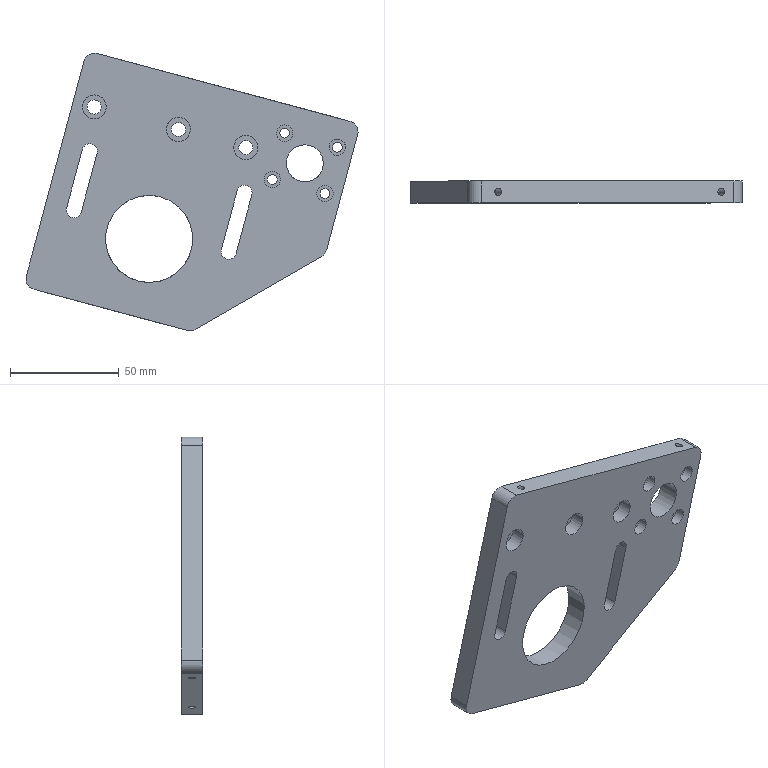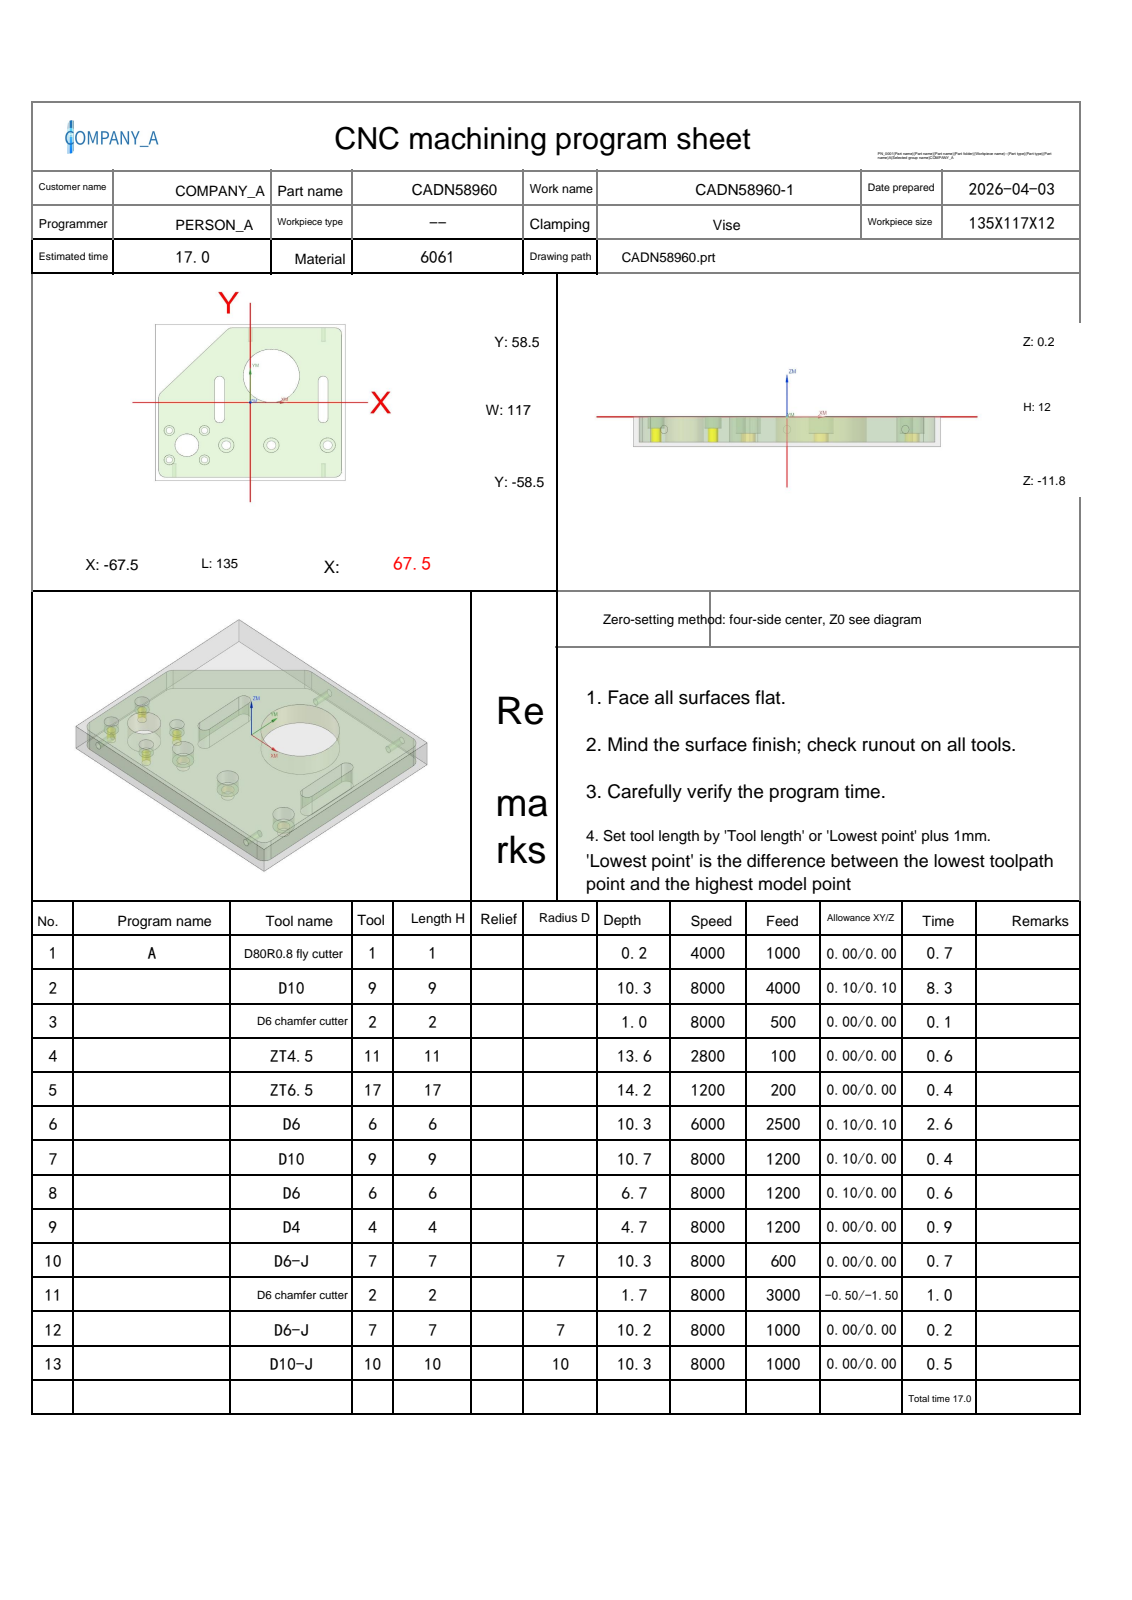NC program | NX | posted by the shop | part box 152.311 x 10 x 127.359 mm
Lines 3046 to 4827 of 4827, first 1275 of 1782 lines:
N3 T02 M06
(D6 chamfer cutter  D=6. R=0. H=02 ce=0.00 di=0.10)
G00 G90 G54 X15. Y19.989 M03 S8000
G43 H02 Z20.
M08
G98 G82 X15. Y19.989 Z-.8 R1. F500.
G80
G00 Z20.
G00 G90 X55. Y-32. M03 S8000
Z20.
G98 G81 X55. Y-32. Z-.8 R1. F500.
X15.
X-17.
X-32.5 Y-21.
Y-43.
X-45. Y-32.
X-57.5 Y-21.
Y-43.
G80
G00 Z20.
G91 G28 Z0.0
M05
M09
G91 G28 Z0.0
M01
N4 T11 M06
(ZT4.5 D=4.5 DR_a=118 H=11)
G00 G90 G54 X-57.5 Y-21. M03 S2800
G43 H11 Z20.
M08
G98 G83 X-57.5 Y-21. Z-13.352 R1. F100. Q2.
Y-43.
X-32.5
Y-21.
G80
G00 Z20.
G91 G28 Z0.0
M05
M09
G91 G28 Z0.0
M01
N5 T17 M06
(ZT6.5 D=6.5 DR_a=118 H=17)
G00 G90 G54 X55. Y-32. M03 S1200
G43 H17 Z20.
M08
G98 G83 X55. Y-32. Z-13.953 R1. F150. Q2.
X15.
X-17.
G80
G00 Z20.
G00 G90 X-45. Y-32. M03 S800
Z20.
G98 G83 X-45. Y-32. Z-13.953 R1. F200. Q3.
G80
G00 Z20.
G91 G28 Z0.0
M05
M09
G91 G28 Z0.0
M01
N6 T06 M06
(D6  D=6. R=0. H=06 ce=0.10 di=0.10)
G00 G90 G54 X51.37 Y2.219 M03 S6000
G43 H06 Z20.
M08
Z.5
G01 Y-11.781 Z.453 F2500.
G03 X51.77 Y-12.181 Z.451 I.4 J0.0
X52.169 Y-11.781 Z.449 I0.0 J.4
G01 Y16.219 Z.355
G03 X51.875 Y16.605 Z.353 I-.4 J0.0
G01 X51.824 Y16.625
X51.77 Y16.619
G03 X51.37 Y16.219 Z.351 I0.0 J-.4
G01 Y-11.781 Z.257
G03 X51.77 Y-12.181 Z.255 I.4 J0.0
X52.169 Y-11.781 Z.253 I0.0 J.4
G01 Y16.219 Z.159
G03 X51.875 Y16.605 Z.157 I-.4 J0.0
G01 X51.824 Y16.625
X51.77 Y16.619 Z.156
G03 X51.37 Y16.219 Z.154 I0.0 J-.4
G01 Y-11.781 Z.06
G03 X51.77 Y-12.181 Z.058 I.4 J0.0
X52.169 Y-11.781 Z.056 I0.0 J.4
G01 Y16.219 Z-.038
G03 X51.875 Y16.605 Z-.039 I-.4 J0.0
G01 X51.824 Y16.625 Z-.04
X51.77 Y16.619
G03 X51.37 Y16.219 Z-.042 I0.0 J-.4
G01 Y-11.781 Z-.136
G03 X51.77 Y-12.181 Z-.138 I.4 J0.0
X52.169 Y-11.781 Z-.14 I0.0 J.4
G01 Y16.219 Z-.234
G03 X51.875 Y16.605 Z-.236 I-.4 J0.0
G01 X51.824 Y16.625
X51.77 Y16.619
G03 X51.37 Y16.219 Z-.238 I0.0 J-.4
G01 Y-11.781 Z-.332
G03 X51.77 Y-12.181 Z-.334 I.4 J0.0
X52.169 Y-11.781 Z-.336 I0.0 J.4
G01 Y16.219 Z-.43
G03 X51.875 Y16.605 Z-.432 I-.4 J0.0
G01 X51.824 Y16.625
X51.77 Y16.619
G03 X51.37 Y16.219 Z-.435 I0.0 J-.4
G01 Y-11.781 Z-.528
G03 X51.77 Y-12.181 Z-.531 I.4 J0.0
X52.169 Y-11.781 Z-.533 I0.0 J.4
G01 Y16.219 Z-.627
G03 X51.875 Y16.605 Z-.628 I-.4 J0.0
G01 X51.824 Y16.625 Z-.629
X51.77 Y16.619
G03 X51.37 Y16.219 Z-.631 I0.0 J-.4
G01 Y-11.781 Z-.725
G03 X51.77 Y-12.181 Z-.727 I.4 J0.0
X52.169 Y-11.781 Z-.729 I0.0 J.4
G01 Y16.219 Z-.823
G03 X51.875 Y16.605 Z-.825 I-.4 J0.0
G01 X51.824 Y16.625
X51.77 Y16.619
G03 X51.37 Y16.219 Z-.827 I0.0 J-.4
G01 Y-11.781 Z-.921
G03 X51.77 Y-12.181 Z-.923 I.4 J0.0
X52.169 Y-11.781 Z-.925 I0.0 J.4
G01 Y16.219 Z-1.019
G03 X51.875 Y16.605 Z-1.021 I-.4 J0.0
G01 X51.824 Y16.625
X51.77 Y16.619
G03 X51.37 Y16.219 Z-1.023 I0.0 J-.4
G01 Y-11.781 Z-1.117
G03 X51.77 Y-12.181 Z-1.119 I.4 J0.0
X52.169 Y-11.781 Z-1.122 I0.0 J.4
G01 Y16.219 Z-1.215
G03 X51.875 Y16.605 Z-1.217 I-.4 J0.0
G01 X51.824 Y16.625
X51.77 Y16.619 Z-1.218
G03 X51.37 Y16.219 Z-1.22 I0.0 J-.4
G01 Y-11.781 Z-1.314
G03 X51.77 Y-12.181 Z-1.316 I.4 J0.0
X52.169 Y-11.781 Z-1.318 I0.0 J.4
G01 Y16.219 Z-1.412
G03 X51.875 Y16.605 Z-1.414 I-.4 J0.0
G01 X51.824 Y16.625
X51.77 Y16.619
G03 X51.37 Y16.219 Z-1.416 I0.0 J-.4
G01 Y-11.781 Z-1.51
G03 X51.77 Y-12.181 Z-1.512 I.4 J0.0
X52.169 Y-11.781 Z-1.514 I0.0 J.4
G01 Y16.219 Z-1.608
G03 X51.875 Y16.605 Z-1.61 I-.4 J0.0
G01 X51.824 Y16.625
X51.77 Y16.619
G03 X51.37 Y16.219 Z-1.612 I0.0 J-.4
G01 Y-11.781 Z-1.706
G03 X51.77 Y-12.181 Z-1.708 I.4 J0.0
X52.169 Y-11.781 Z-1.71 I0.0 J.4
G01 Y16.219 Z-1.804
G03 X51.875 Y16.605 Z-1.806 I-.4 J0.0
G01 X51.824 Y16.625
X51.77 Y16.619
G03 X51.37 Y16.219 Z-1.809 I0.0 J-.4
G01 Y-11.781 Z-1.903
G03 X51.77 Y-12.181 Z-1.905 I.4 J0.0
X52.169 Y-11.781 Z-1.907 I0.0 J.4
G01 Y16.219 Z-2.001
G03 X51.875 Y16.605 Z-2.002 I-.4 J0.0
G01 X51.824 Y16.625 Z-2.003
X51.77 Y16.619
G03 X51.37 Y16.219 Z-2.005 I0.0 J-.4
G01 Y-11.781 Z-2.099
G03 X51.77 Y-12.181 Z-2.101 I.4 J0.0
X52.169 Y-11.781 Z-2.103 I0.0 J.4
G01 Y16.219 Z-2.197
G03 X51.875 Y16.605 Z-2.199 I-.4 J0.0
G01 X51.824 Y16.625
X51.77 Y16.619
G03 X51.37 Y16.219 Z-2.201 I0.0 J-.4
G01 Y-11.781 Z-2.295
G03 X51.77 Y-12.181 Z-2.297 I.4 J0.0
X52.169 Y-11.781 Z-2.299 I0.0 J.4
G01 Y16.219 Z-2.393
G03 X51.875 Y16.605 Z-2.395 I-.4 J0.0
G01 X51.824 Y16.625
X51.77 Y16.619
G03 X51.37 Y16.219 Z-2.397 I0.0 J-.4
G01 Y-11.781 Z-2.491
G03 X51.77 Y-12.181 Z-2.494 I.4 J0.0
X52.169 Y-11.781 Z-2.496 I0.0 J.4
G01 Y16.219 Z-2.59
G03 X51.875 Y16.605 Z-2.591 I-.4 J0.0
G01 X51.824 Y16.625
X51.77 Y16.619 Z-2.592
G03 X51.37 Y16.219 Z-2.594 I0.0 J-.4
G01 Y-11.781 Z-2.688
G03 X51.77 Y-12.181 Z-2.69 I.4 J0.0
X52.169 Y-11.781 Z-2.692 I0.0 J.4
G01 Y16.219 Z-2.786
G03 X51.875 Y16.605 Z-2.788 I-.4 J0.0
G01 X51.824 Y16.625
X51.77 Y16.619
G03 X51.37 Y16.219 Z-2.79 I0.0 J-.4
G01 Y-11.781 Z-2.884
G03 X51.77 Y-12.181 Z-2.886 I.4 J0.0
X52.169 Y-11.781 Z-2.888 I0.0 J.4
G01 Y16.219 Z-2.982
G03 X51.875 Y16.605 Z-2.984 I-.4 J0.0
G01 X51.824 Y16.625
X51.77 Y16.619
G03 X51.37 Y16.219 Z-2.986 I0.0 J-.4
G01 Y-11.781 Z-3.08
G03 X51.77 Y-12.181 Z-3.082 I.4 J0.0
X52.169 Y-11.781 Z-3.085 I0.0 J.4
G01 Y16.219 Z-3.178
G03 X51.875 Y16.605 Z-3.18 I-.4 J0.0
G01 X51.824 Y16.625
X51.77 Y16.619 Z-3.181
G03 X51.37 Y16.219 Z-3.183 I0.0 J-.4
G01 Y-11.781 Z-3.277
G03 X51.77 Y-12.181 Z-3.279 I.4 J0.0
X52.169 Y-11.781 Z-3.281 I0.0 J.4
G01 Y16.219 Z-3.375
G03 X51.875 Y16.605 Z-3.376 I-.4 J0.0
G01 X51.824 Y16.625 Z-3.377
X51.77 Y16.619
G03 X51.37 Y16.219 Z-3.379 I0.0 J-.4
G01 Y-11.781 Z-3.473
G03 X51.77 Y-12.181 Z-3.475 I.4 J0.0
X52.169 Y-11.781 Z-3.477 I0.0 J.4
G01 Y16.219 Z-3.571
G03 X51.875 Y16.605 Z-3.573 I-.4 J0.0
G01 X51.824 Y16.625
X51.77 Y16.619
G03 X51.37 Y16.219 Z-3.575 I0.0 J-.4
G01 Y-11.781 Z-3.669
G03 X51.77 Y-12.181 Z-3.671 I.4 J0.0
X52.169 Y-11.781 Z-3.673 I0.0 J.4
G01 Y16.219 Z-3.767
G03 X51.875 Y16.605 Z-3.769 I-.4 J0.0
G01 X51.824 Y16.625
X51.77 Y16.619
G03 X51.37 Y16.219 Z-3.772 I0.0 J-.4
G01 Y-11.781 Z-3.865
G03 X51.77 Y-12.181 Z-3.868 I.4 J0.0
X52.169 Y-11.781 Z-3.87 I0.0 J.4
G01 Y16.219 Z-3.964
G03 X51.875 Y16.605 Z-3.965 I-.4 J0.0
G01 X51.824 Y16.625 Z-3.966
X51.77 Y16.619
G03 X51.37 Y16.219 Z-3.968 I0.0 J-.4
G01 Y-11.781 Z-4.062
G03 X51.77 Y-12.181 Z-4.064 I.4 J0.0
X52.169 Y-11.781 Z-4.066 I0.0 J.4
G01 Y16.219 Z-4.16
G03 X51.875 Y16.605 Z-4.162 I-.4 J0.0
G01 X51.824 Y16.625
X51.77 Y16.619
G03 X51.37 Y16.219 Z-4.164 I0.0 J-.4
G01 Y-11.781 Z-4.258
G03 X51.77 Y-12.181 Z-4.26 I.4 J0.0
X52.169 Y-11.781 Z-4.262 I0.0 J.4
G01 Y16.219 Z-4.356
G03 X51.875 Y16.605 Z-4.358 I-.4 J0.0
G01 X51.824 Y16.625
X51.77 Y16.619
G03 X51.37 Y16.219 Z-4.36 I0.0 J-.4
G01 Y-11.781 Z-4.454
G03 X51.77 Y-12.181 Z-4.456 I.4 J0.0
X52.169 Y-11.781 Z-4.459 I0.0 J.4
G01 Y16.219 Z-4.553
G03 X51.875 Y16.605 Z-4.554 I-.4 J0.0
G01 X51.824 Y16.625
X51.77 Y16.619 Z-4.555
G03 X51.37 Y16.219 Z-4.557 I0.0 J-.4
G01 Y-11.781 Z-4.651
G03 X51.77 Y-12.181 Z-4.653 I.4 J0.0
X52.169 Y-11.781 Z-4.655 I0.0 J.4
G01 Y16.219 Z-4.749
G03 X51.875 Y16.605 Z-4.751 I-.4 J0.0
G01 X51.824 Y16.625
X51.77 Y16.619
G03 X51.37 Y16.219 Z-4.753 I0.0 J-.4
G01 Y-11.781 Z-4.847
G03 X51.77 Y-12.181 Z-4.849 I.4 J0.0
X52.169 Y-11.781 Z-4.851 I0.0 J.4
G01 Y16.219 Z-4.945
G03 X51.875 Y16.605 Z-4.947 I-.4 J0.0
G01 X51.824 Y16.625
X51.77 Y16.619
G03 X51.37 Y16.219 Z-4.949 I0.0 J-.4
G01 Y-11.781 Z-5.043
G03 X51.77 Y-12.181 Z-5.045 I.4 J0.0
X52.169 Y-11.781 Z-5.047 I0.0 J.4
G01 Y16.219 Z-5.141
G03 X51.875 Y16.605 Z-5.143 I-.4 J0.0
G01 X51.824 Y16.625
X51.77 Y16.619 Z-5.144
G03 X51.37 Y16.219 Z-5.146 I0.0 J-.4
G01 Y-11.781 Z-5.24
G03 X51.77 Y-12.181 Z-5.242 I.4 J0.0
X52.169 Y-11.781 Z-5.244 I0.0 J.4
G01 Y16.219 Z-5.338
G03 X51.875 Y16.605 Z-5.339 I-.4 J0.0
G01 X51.824 Y16.625 Z-5.34
X51.77 Y16.619
G03 X51.37 Y16.219 Z-5.342 I0.0 J-.4
G01 Y-11.781 Z-5.436
G03 X51.77 Y-12.181 Z-5.438 I.4 J0.0
X52.169 Y-11.781 Z-5.44 I0.0 J.4
G01 Y16.219 Z-5.534
G03 X51.875 Y16.605 Z-5.536 I-.4 J0.0
G01 X51.824 Y16.625
X51.77 Y16.619
G03 X51.37 Y16.219 Z-5.538 I0.0 J-.4
G01 Y-11.781 Z-5.632
G03 X51.77 Y-12.181 Z-5.634 I.4 J0.0
X52.169 Y-11.781 Z-5.636 I0.0 J.4
G01 Y16.219 Z-5.73
G03 X51.875 Y16.605 Z-5.732 I-.4 J0.0
G01 X51.824 Y16.625
X51.77 Y16.619
G03 X51.37 Y16.219 Z-5.735 I0.0 J-.4
G01 Y-11.781 Z-5.828
G03 X51.77 Y-12.181 Z-5.831 I.4 J0.0
X52.169 Y-11.781 Z-5.833 I0.0 J.4
G01 Y16.219 Z-5.927
G03 X51.875 Y16.605 Z-5.928 I-.4 J0.0
G01 X51.824 Y16.625 Z-5.929
X51.77 Y16.619
G03 X51.37 Y16.219 Z-5.931 I0.0 J-.4
G01 Y-11.781 Z-6.025
G03 X51.77 Y-12.181 Z-6.027 I.4 J0.0
X52.169 Y-11.781 Z-6.029 I0.0 J.4
G01 Y16.219 Z-6.123
G03 X51.875 Y16.605 Z-6.125 I-.4 J0.0
G01 X51.824 Y16.625
X51.77 Y16.619
G03 X51.37 Y16.219 Z-6.127 I0.0 J-.4
G01 Y-11.781 Z-6.221
G03 X51.77 Y-12.181 Z-6.223 I.4 J0.0
X52.169 Y-11.781 Z-6.225 I0.0 J.4
G01 Y16.219 Z-6.319
G03 X51.875 Y16.605 Z-6.321 I-.4 J0.0
G01 X51.824 Y16.625
X51.77 Y16.619
G03 X51.37 Y16.219 Z-6.323 I0.0 J-.4
G01 Y-11.781 Z-6.417
G03 X51.77 Y-12.181 Z-6.419 I.4 J0.0
X52.169 Y-11.781 Z-6.422 I0.0 J.4
G01 Y16.219 Z-6.515
G03 X51.875 Y16.605 Z-6.517 I-.4 J0.0
G01 X51.824 Y16.625
X51.77 Y16.619 Z-6.518
G03 X51.37 Y16.219 Z-6.52 I0.0 J-.4
G01 Y-11.781 Z-6.614
G03 X51.77 Y-12.181 Z-6.616 I.4 J0.0
X52.169 Y-11.781 Z-6.618 I0.0 J.4
G01 Y16.219 Z-6.712
G03 X51.875 Y16.605 Z-6.714 I-.4 J0.0
G01 X51.824 Y16.625
X51.77 Y16.619
G03 X51.37 Y16.219 Z-6.716 I0.0 J-.4
G01 Y-11.781 Z-6.81
G03 X51.77 Y-12.181 Z-6.812 I.4 J0.0
X52.169 Y-11.781 Z-6.814 I0.0 J.4
G01 Y16.219 Z-6.908
G03 X51.875 Y16.605 Z-6.91 I-.4 J0.0
G01 X51.824 Y16.625
X51.77 Y16.619
G03 X51.37 Y16.219 Z-6.912 I0.0 J-.4
G01 Y-11.781 Z-7.006
G03 X51.77 Y-12.181 Z-7.008 I.4 J0.0
X52.169 Y-11.781 Z-7.01 I0.0 J.4
G01 Y16.219 Z-7.104
G03 X51.875 Y16.605 Z-7.106 I-.4 J0.0
G01 X51.824 Y16.625
X51.77 Y16.619
G03 X51.37 Y16.219 Z-7.109 I0.0 J-.4
G01 Y-11.781 Z-7.203
G03 X51.77 Y-12.181 Z-7.205 I.4 J0.0
X52.169 Y-11.781 Z-7.207 I0.0 J.4
G01 Y16.219 Z-7.301
G03 X51.875 Y16.605 Z-7.302 I-.4 J0.0
G01 X51.824 Y16.625 Z-7.303
X51.77 Y16.619
G03 X51.37 Y16.219 Z-7.305 I0.0 J-.4
G01 Y-11.781 Z-7.399
G03 X51.77 Y-12.181 Z-7.401 I.4 J0.0
X52.169 Y-11.781 Z-7.403 I0.0 J.4
G01 Y16.219 Z-7.497
G03 X51.875 Y16.605 Z-7.499 I-.4 J0.0
G01 X51.824 Y16.625
X51.77 Y16.619
G03 X51.37 Y16.219 Z-7.501 I0.0 J-.4
G01 Y-11.781 Z-7.595
G03 X51.77 Y-12.181 Z-7.597 I.4 J0.0
X52.169 Y-11.781 Z-7.599 I0.0 J.4
G01 Y16.219 Z-7.693
G03 X51.875 Y16.605 Z-7.695 I-.4 J0.0
G01 X51.824 Y16.625
X51.77 Y16.619
G03 X51.37 Y16.219 Z-7.697 I0.0 J-.4
G01 Y-11.781 Z-7.791
G03 X51.77 Y-12.181 Z-7.794 I.4 J0.0
X52.169 Y-11.781 Z-7.796 I0.0 J.4
G01 Y16.219 Z-7.89
G03 X51.875 Y16.605 Z-7.891 I-.4 J0.0
G01 X51.824 Y16.625
X51.77 Y16.619 Z-7.892
G03 X51.37 Y16.219 Z-7.894 I0.0 J-.4
G01 Y-11.781 Z-7.988
G03 X51.77 Y-12.181 Z-7.99 I.4 J0.0
X52.169 Y-11.781 Z-7.992 I0.0 J.4
G01 Y16.219 Z-8.086
G03 X51.875 Y16.605 Z-8.088 I-.4 J0.0
G01 X51.824 Y16.625
X51.77 Y16.619
G03 X51.37 Y16.219 Z-8.09 I0.0 J-.4
G01 Y-11.781 Z-8.184
G03 X51.77 Y-12.181 Z-8.186 I.4 J0.0
X52.169 Y-11.781 Z-8.188 I0.0 J.4
G01 Y16.219 Z-8.282
G03 X51.875 Y16.605 Z-8.284 I-.4 J0.0
G01 X51.824 Y16.625
X51.77 Y16.619
G03 X51.37 Y16.219 Z-8.286 I0.0 J-.4
G01 Y-11.781 Z-8.38
G03 X51.77 Y-12.181 Z-8.382 I.4 J0.0
X52.169 Y-11.781 Z-8.385 I0.0 J.4
G01 Y16.219 Z-8.478
G03 X51.875 Y16.605 Z-8.48 I-.4 J0.0
G01 X51.824 Y16.625
X51.77 Y16.619 Z-8.481
G03 X51.37 Y16.219 Z-8.483 I0.0 J-.4
G01 Y-11.781 Z-8.577
G03 X51.77 Y-12.181 Z-8.579 I.4 J0.0
X52.169 Y-11.781 Z-8.581 I0.0 J.4
G01 Y16.219 Z-8.675
G03 X51.875 Y16.605 Z-8.676 I-.4 J0.0
G01 X51.824 Y16.625 Z-8.677
X51.77 Y16.619
G03 X51.37 Y16.219 Z-8.679 I0.0 J-.4
G01 Y-11.781 Z-8.773
G03 X51.77 Y-12.181 Z-8.775 I.4 J0.0
X52.169 Y-11.781 Z-8.777 I0.0 J.4
G01 Y16.219 Z-8.871
G03 X51.875 Y16.605 Z-8.873 I-.4 J0.0
G01 X51.824 Y16.625
X51.77 Y16.619
G03 X51.37 Y16.219 Z-8.875 I0.0 J-.4
G01 Y-11.781 Z-8.969
G03 X51.77 Y-12.181 Z-8.971 I.4 J0.0
X52.169 Y-11.781 Z-8.973 I0.0 J.4
G01 Y16.219 Z-9.067
G03 X51.875 Y16.605 Z-9.069 I-.4 J0.0
G01 X51.824 Y16.625
X51.77 Y16.619
G03 X51.37 Y16.219 Z-9.072 I0.0 J-.4
G01 Y-11.781 Z-9.165
G03 X51.77 Y-12.181 Z-9.168 I.4 J0.0
X52.169 Y-11.781 Z-9.17 I0.0 J.4
G01 Y16.219 Z-9.264
G03 X51.875 Y16.605 Z-9.265 I-.4 J0.0
G01 X51.824 Y16.625 Z-9.266
X51.77 Y16.619
G03 X51.37 Y16.219 Z-9.268 I0.0 J-.4
G01 Y-11.781 Z-9.362
G03 X51.77 Y-12.181 Z-9.364 I.4 J0.0
X52.169 Y-11.781 Z-9.366 I0.0 J.4
G01 Y16.219 Z-9.46
G03 X51.875 Y16.605 Z-9.462 I-.4 J0.0
G01 X51.824 Y16.625
X51.77 Y16.619
G03 X51.37 Y16.219 Z-9.464 I0.0 J-.4
G01 Y-11.781 Z-9.558
G03 X51.77 Y-12.181 Z-9.56 I.4 J0.0
X52.169 Y-11.781 Z-9.562 I0.0 J.4
G01 Y16.219 Z-9.656
G03 X51.875 Y16.605 Z-9.658 I-.4 J0.0
G01 X51.824 Y16.625
X51.77 Y16.619
G03 X51.37 Y16.219 Z-9.66 I0.0 J-.4
G01 Y-11.781 Z-9.754
G03 X51.77 Y-12.181 Z-9.756 I.4 J0.0
X52.169 Y-11.781 Z-9.759 I0.0 J.4
G01 Y16.219 Z-9.853
G03 X51.875 Y16.605 Z-9.854 I-.4 J0.0
G01 X51.824 Y16.625
X51.77 Y16.619 Z-9.855
G03 X51.37 Y16.219 Z-9.857 I0.0 J-.4
G01 Y-11.781 Z-9.951
G03 X51.77 Y-12.181 Z-9.953 I.4 J0.0
X52.169 Y-11.781 Z-9.955 I0.0 J.4
G01 Y16.219 Z-10.049
G03 X51.875 Y16.605 Z-10.051 I-.4 J0.0
G01 X51.824 Y16.625
X51.77 Y16.619
G03 X51.37 Y16.219 Z-10.053 I0.0 J-.4
G01 Y2.219 Z-10.1
Y-11.781
G03 X51.77 Y-12.181 I.4 J0.0
X52.169 Y-11.781 I0.0 J.4
G01 Y16.219
G03 X51.77 Y16.619 I-.4 J0.0
X51.37 Y16.219 I0.0 J-.4
G01 Y2.219
Y1.719
Z-9.1
G00 Z20.
X-22.169 Y2.219
Z.5
G01 Y-11.781 Z.453
G03 X-21.77 Y-12.181 Z.451 I.4 J0.0
X-21.37 Y-11.781 Z.449 I0.0 J.4
G01 Y16.219 Z.355
G03 X-21.77 Y16.619 Z.353 I-.4 J0.0
X-22.169 Y16.219 Z.351 I0.0 J-.4
G01 Y-11.781 Z.257
G03 X-21.77 Y-12.181 Z.255 I.4 J0.0
X-21.37 Y-11.781 Z.253 I0.0 J.4
G01 Y16.219 Z.159
G03 X-21.77 Y16.619 Z.156 I-.4 J0.0
X-22.169 Y16.219 Z.154 I0.0 J-.4
G01 Y-11.781 Z.06
G03 X-21.77 Y-12.181 Z.058 I.4 J0.0
X-21.37 Y-11.781 Z.056 I0.0 J.4
G01 Y16.219 Z-.038
G03 X-21.77 Y16.619 Z-.04 I-.4 J0.0
X-22.169 Y16.219 Z-.042 I0.0 J-.4
G01 Y-11.781 Z-.136
G03 X-21.77 Y-12.181 Z-.138 I.4 J0.0
X-21.37 Y-11.781 Z-.14 I0.0 J.4
G01 Y16.219 Z-.234
G03 X-21.77 Y16.619 Z-.236 I-.4 J0.0
X-22.169 Y16.219 Z-.238 I0.0 J-.4
G01 Y-11.781 Z-.332
G03 X-21.77 Y-12.181 Z-.334 I.4 J0.0
X-21.37 Y-11.781 Z-.336 I0.0 J.4
G01 Y16.219 Z-.43
G03 X-21.77 Y16.619 Z-.432 I-.4 J0.0
X-22.169 Y16.219 Z-.435 I0.0 J-.4
G01 Y-11.781 Z-.528
G03 X-21.77 Y-12.181 Z-.531 I.4 J0.0
X-21.37 Y-11.781 Z-.533 I0.0 J.4
G01 Y16.219 Z-.627
G03 X-21.77 Y16.619 Z-.629 I-.4 J0.0
X-22.169 Y16.219 Z-.631 I0.0 J-.4
G01 Y-11.781 Z-.725
G03 X-21.77 Y-12.181 Z-.727 I.4 J0.0
X-21.37 Y-11.781 Z-.729 I0.0 J.4
G01 Y16.219 Z-.823
G03 X-21.77 Y16.619 Z-.825 I-.4 J0.0
X-22.169 Y16.219 Z-.827 I0.0 J-.4
G01 Y-11.781 Z-.921
G03 X-21.77 Y-12.181 Z-.923 I.4 J0.0
X-21.37 Y-11.781 Z-.925 I0.0 J.4
G01 Y16.219 Z-1.019
G03 X-21.77 Y16.619 Z-1.021 I-.4 J0.0
X-22.169 Y16.219 Z-1.023 I0.0 J-.4
G01 Y-11.781 Z-1.117
G03 X-21.77 Y-12.181 Z-1.119 I.4 J0.0
X-21.37 Y-11.781 Z-1.122 I0.0 J.4
G01 Y16.219 Z-1.215
G03 X-21.77 Y16.619 Z-1.218 I-.4 J0.0
X-22.169 Y16.219 Z-1.22 I0.0 J-.4
G01 Y-11.781 Z-1.314
G03 X-21.77 Y-12.181 Z-1.316 I.4 J0.0
X-21.37 Y-11.781 Z-1.318 I0.0 J.4
G01 Y16.219 Z-1.412
G03 X-21.77 Y16.619 Z-1.414 I-.4 J0.0
X-22.169 Y16.219 Z-1.416 I0.0 J-.4
G01 Y-11.781 Z-1.51
G03 X-21.77 Y-12.181 Z-1.512 I.4 J0.0
X-21.37 Y-11.781 Z-1.514 I0.0 J.4
G01 Y16.219 Z-1.608
G03 X-21.77 Y16.619 Z-1.61 I-.4 J0.0
X-22.169 Y16.219 Z-1.612 I0.0 J-.4
G01 Y-11.781 Z-1.706
G03 X-21.77 Y-12.181 Z-1.708 I.4 J0.0
X-21.37 Y-11.781 Z-1.71 I0.0 J.4
G01 Y16.219 Z-1.804
G03 X-21.77 Y16.619 Z-1.806 I-.4 J0.0
X-22.169 Y16.219 Z-1.809 I0.0 J-.4
G01 Y-11.781 Z-1.903
G03 X-21.77 Y-12.181 Z-1.905 I.4 J0.0
X-21.37 Y-11.781 Z-1.907 I0.0 J.4
G01 Y16.219 Z-2.001
G03 X-21.77 Y16.619 Z-2.003 I-.4 J0.0
X-22.169 Y16.219 Z-2.005 I0.0 J-.4
G01 Y-11.781 Z-2.099
G03 X-21.77 Y-12.181 Z-2.101 I.4 J0.0
X-21.37 Y-11.781 Z-2.103 I0.0 J.4
G01 Y16.219 Z-2.197
G03 X-21.77 Y16.619 Z-2.199 I-.4 J0.0
X-22.169 Y16.219 Z-2.201 I0.0 J-.4
G01 Y-11.781 Z-2.295
G03 X-21.77 Y-12.181 Z-2.297 I.4 J0.0
X-21.37 Y-11.781 Z-2.299 I0.0 J.4
G01 Y16.219 Z-2.393
G03 X-21.77 Y16.619 Z-2.395 I-.4 J0.0
X-22.169 Y16.219 Z-2.397 I0.0 J-.4
G01 Y-11.781 Z-2.491
G03 X-21.77 Y-12.181 Z-2.494 I.4 J0.0
X-21.37 Y-11.781 Z-2.496 I0.0 J.4
G01 Y16.219 Z-2.59
G03 X-21.77 Y16.619 Z-2.592 I-.4 J0.0
X-22.169 Y16.219 Z-2.594 I0.0 J-.4
G01 Y-11.781 Z-2.688
G03 X-21.77 Y-12.181 Z-2.69 I.4 J0.0
X-21.37 Y-11.781 Z-2.692 I0.0 J.4
G01 Y16.219 Z-2.786
G03 X-21.77 Y16.619 Z-2.788 I-.4 J0.0
X-22.169 Y16.219 Z-2.79 I0.0 J-.4
G01 Y-11.781 Z-2.884
G03 X-21.77 Y-12.181 Z-2.886 I.4 J0.0
X-21.37 Y-11.781 Z-2.888 I0.0 J.4
G01 Y16.219 Z-2.982
G03 X-21.77 Y16.619 Z-2.984 I-.4 J0.0
X-22.169 Y16.219 Z-2.986 I0.0 J-.4
G01 Y-11.781 Z-3.08
G03 X-21.77 Y-12.181 Z-3.082 I.4 J0.0
X-21.37 Y-11.781 Z-3.085 I0.0 J.4
G01 Y16.219 Z-3.178
G03 X-21.77 Y16.619 Z-3.181 I-.4 J0.0
X-22.169 Y16.219 Z-3.183 I0.0 J-.4
G01 Y-11.781 Z-3.277
G03 X-21.77 Y-12.181 Z-3.279 I.4 J0.0
X-21.37 Y-11.781 Z-3.281 I0.0 J.4
G01 Y16.219 Z-3.375
G03 X-21.77 Y16.619 Z-3.377 I-.4 J0.0
X-22.169 Y16.219 Z-3.379 I0.0 J-.4
G01 Y-11.781 Z-3.473
G03 X-21.77 Y-12.181 Z-3.475 I.4 J0.0
X-21.37 Y-11.781 Z-3.477 I0.0 J.4
G01 Y16.219 Z-3.571
G03 X-21.77 Y16.619 Z-3.573 I-.4 J0.0
X-22.169 Y16.219 Z-3.575 I0.0 J-.4
G01 Y-11.781 Z-3.669
G03 X-21.77 Y-12.181 Z-3.671 I.4 J0.0
X-21.37 Y-11.781 Z-3.673 I0.0 J.4
G01 Y16.219 Z-3.767
G03 X-21.77 Y16.619 Z-3.769 I-.4 J0.0
X-22.169 Y16.219 Z-3.772 I0.0 J-.4
G01 Y-11.781 Z-3.865
G03 X-21.77 Y-12.181 Z-3.868 I.4 J0.0
X-21.37 Y-11.781 Z-3.87 I0.0 J.4
G01 Y16.219 Z-3.964
G03 X-21.77 Y16.619 Z-3.966 I-.4 J0.0
X-22.169 Y16.219 Z-3.968 I0.0 J-.4
G01 Y-11.781 Z-4.062
G03 X-21.77 Y-12.181 Z-4.064 I.4 J0.0
X-21.37 Y-11.781 Z-4.066 I0.0 J.4
G01 Y16.219 Z-4.16
G03 X-21.77 Y16.619 Z-4.162 I-.4 J0.0
X-22.169 Y16.219 Z-4.164 I0.0 J-.4
G01 Y-11.781 Z-4.258
G03 X-21.77 Y-12.181 Z-4.26 I.4 J0.0
X-21.37 Y-11.781 Z-4.262 I0.0 J.4
G01 Y16.219 Z-4.356
G03 X-21.77 Y16.619 Z-4.358 I-.4 J0.0
X-22.169 Y16.219 Z-4.36 I0.0 J-.4
G01 Y-11.781 Z-4.454
G03 X-21.77 Y-12.181 Z-4.456 I.4 J0.0
X-21.37 Y-11.781 Z-4.459 I0.0 J.4
G01 Y16.219 Z-4.553
G03 X-21.77 Y16.619 Z-4.555 I-.4 J0.0
X-22.169 Y16.219 Z-4.557 I0.0 J-.4
G01 Y-11.781 Z-4.651
G03 X-21.77 Y-12.181 Z-4.653 I.4 J0.0
X-21.37 Y-11.781 Z-4.655 I0.0 J.4
G01 Y16.219 Z-4.749
G03 X-21.77 Y16.619 Z-4.751 I-.4 J0.0
X-22.169 Y16.219 Z-4.753 I0.0 J-.4
G01 Y-11.781 Z-4.847
G03 X-21.77 Y-12.181 Z-4.849 I.4 J0.0
X-21.37 Y-11.781 Z-4.851 I0.0 J.4
G01 Y16.219 Z-4.945
G03 X-21.77 Y16.619 Z-4.947 I-.4 J0.0
X-22.169 Y16.219 Z-4.949 I0.0 J-.4
G01 Y-11.781 Z-5.043
G03 X-21.77 Y-12.181 Z-5.045 I.4 J0.0
X-21.37 Y-11.781 Z-5.047 I0.0 J.4
G01 Y16.219 Z-5.141
G03 X-21.77 Y16.619 Z-5.144 I-.4 J0.0
X-22.169 Y16.219 Z-5.146 I0.0 J-.4
G01 Y-11.781 Z-5.24
G03 X-21.77 Y-12.181 Z-5.242 I.4 J0.0
X-21.37 Y-11.781 Z-5.244 I0.0 J.4
G01 Y16.219 Z-5.338
G03 X-21.77 Y16.619 Z-5.34 I-.4 J0.0
X-22.169 Y16.219 Z-5.342 I0.0 J-.4
G01 Y-11.781 Z-5.436
G03 X-21.77 Y-12.181 Z-5.438 I.4 J0.0
X-21.37 Y-11.781 Z-5.44 I0.0 J.4
G01 Y16.219 Z-5.534
G03 X-21.77 Y16.619 Z-5.536 I-.4 J0.0
X-22.169 Y16.219 Z-5.538 I0.0 J-.4
G01 Y-11.781 Z-5.632
G03 X-21.77 Y-12.181 Z-5.634 I.4 J0.0
X-21.37 Y-11.781 Z-5.636 I0.0 J.4
G01 Y16.219 Z-5.73
G03 X-21.77 Y16.619 Z-5.732 I-.4 J0.0
X-22.169 Y16.219 Z-5.735 I0.0 J-.4
G01 Y-11.781 Z-5.828
G03 X-21.77 Y-12.181 Z-5.831 I.4 J0.0
X-21.37 Y-11.781 Z-5.833 I0.0 J.4
G01 Y16.219 Z-5.927
G03 X-21.77 Y16.619 Z-5.929 I-.4 J0.0
X-22.169 Y16.219 Z-5.931 I0.0 J-.4
G01 Y-11.781 Z-6.025
G03 X-21.77 Y-12.181 Z-6.027 I.4 J0.0
X-21.37 Y-11.781 Z-6.029 I0.0 J.4
G01 Y16.219 Z-6.123
G03 X-21.77 Y16.619 Z-6.125 I-.4 J0.0
X-22.169 Y16.219 Z-6.127 I0.0 J-.4
G01 Y-11.781 Z-6.221
G03 X-21.77 Y-12.181 Z-6.223 I.4 J0.0
X-21.37 Y-11.781 Z-6.225 I0.0 J.4
G01 Y16.219 Z-6.319
G03 X-21.77 Y16.619 Z-6.321 I-.4 J0.0
X-22.169 Y16.219 Z-6.323 I0.0 J-.4
G01 Y-11.781 Z-6.417
G03 X-21.77 Y-12.181 Z-6.419 I.4 J0.0
X-21.37 Y-11.781 Z-6.422 I0.0 J.4
G01 Y16.219 Z-6.515
G03 X-21.77 Y16.619 Z-6.518 I-.4 J0.0
X-22.169 Y16.219 Z-6.52 I0.0 J-.4
G01 Y-11.781 Z-6.614
G03 X-21.77 Y-12.181 Z-6.616 I.4 J0.0
X-21.37 Y-11.781 Z-6.618 I0.0 J.4
G01 Y16.219 Z-6.712
G03 X-21.77 Y16.619 Z-6.714 I-.4 J0.0
X-22.169 Y16.219 Z-6.716 I0.0 J-.4
G01 Y-11.781 Z-6.81
G03 X-21.77 Y-12.181 Z-6.812 I.4 J0.0
X-21.37 Y-11.781 Z-6.814 I0.0 J.4
G01 Y16.219 Z-6.908
G03 X-21.77 Y16.619 Z-6.91 I-.4 J0.0
X-22.169 Y16.219 Z-6.912 I0.0 J-.4
G01 Y-11.781 Z-7.006
G03 X-21.77 Y-12.181 Z-7.008 I.4 J0.0
X-21.37 Y-11.781 Z-7.01 I0.0 J.4
G01 Y16.219 Z-7.104
G03 X-21.77 Y16.619 Z-7.106 I-.4 J0.0
X-22.169 Y16.219 Z-7.109 I0.0 J-.4
G01 Y-11.781 Z-7.203
G03 X-21.77 Y-12.181 Z-7.205 I.4 J0.0
X-21.37 Y-11.781 Z-7.207 I0.0 J.4
G01 Y16.219 Z-7.301
G03 X-21.77 Y16.619 Z-7.303 I-.4 J0.0
X-22.169 Y16.219 Z-7.305 I0.0 J-.4
G01 Y-11.781 Z-7.399
G03 X-21.77 Y-12.181 Z-7.401 I.4 J0.0
X-21.37 Y-11.781 Z-7.403 I0.0 J.4
G01 Y16.219 Z-7.497
G03 X-21.77 Y16.619 Z-7.499 I-.4 J0.0
X-22.169 Y16.219 Z-7.501 I0.0 J-.4
G01 Y-11.781 Z-7.595
G03 X-21.77 Y-12.181 Z-7.597 I.4 J0.0
X-21.37 Y-11.781 Z-7.599 I0.0 J.4
G01 Y16.219 Z-7.693
G03 X-21.77 Y16.619 Z-7.695 I-.4 J0.0
X-22.169 Y16.219 Z-7.697 I0.0 J-.4
G01 Y-11.781 Z-7.791
G03 X-21.77 Y-12.181 Z-7.794 I.4 J0.0
X-21.37 Y-11.781 Z-7.796 I0.0 J.4
G01 Y16.219 Z-7.89
G03 X-21.77 Y16.619 Z-7.892 I-.4 J0.0
X-22.169 Y16.219 Z-7.894 I0.0 J-.4
G01 Y-11.781 Z-7.988
G03 X-21.77 Y-12.181 Z-7.99 I.4 J0.0
X-21.37 Y-11.781 Z-7.992 I0.0 J.4
G01 Y16.219 Z-8.086
G03 X-21.77 Y16.619 Z-8.088 I-.4 J0.0
X-22.169 Y16.219 Z-8.09 I0.0 J-.4
G01 Y-11.781 Z-8.184
G03 X-21.77 Y-12.181 Z-8.186 I.4 J0.0
X-21.37 Y-11.781 Z-8.188 I0.0 J.4
G01 Y16.219 Z-8.282
G03 X-21.77 Y16.619 Z-8.284 I-.4 J0.0
X-22.169 Y16.219 Z-8.286 I0.0 J-.4
G01 Y-11.781 Z-8.38
G03 X-21.77 Y-12.181 Z-8.382 I.4 J0.0
X-21.37 Y-11.781 Z-8.385 I0.0 J.4
G01 Y16.219 Z-8.478
G03 X-21.77 Y16.619 Z-8.481 I-.4 J0.0
X-22.169 Y16.219 Z-8.483 I0.0 J-.4
G01 Y-11.781 Z-8.577
G03 X-21.77 Y-12.181 Z-8.579 I.4 J0.0
X-21.37 Y-11.781 Z-8.581 I0.0 J.4
G01 Y16.219 Z-8.675
G03 X-21.77 Y16.619 Z-8.677 I-.4 J0.0
X-22.169 Y16.219 Z-8.679 I0.0 J-.4
G01 Y-11.781 Z-8.773
G03 X-21.77 Y-12.181 Z-8.775 I.4 J0.0
X-21.37 Y-11.781 Z-8.777 I0.0 J.4
G01 Y16.219 Z-8.871
G03 X-21.77 Y16.619 Z-8.873 I-.4 J0.0
X-22.169 Y16.219 Z-8.875 I0.0 J-.4
G01 Y-11.781 Z-8.969
G03 X-21.77 Y-12.181 Z-8.971 I.4 J0.0
X-21.37 Y-11.781 Z-8.973 I0.0 J.4
G01 Y16.219 Z-9.067
G03 X-21.77 Y16.619 Z-9.069 I-.4 J0.0
X-22.169 Y16.219 Z-9.072 I0.0 J-.4
G01 Y-11.781 Z-9.165
G03 X-21.77 Y-12.181 Z-9.168 I.4 J0.0
X-21.37 Y-11.781 Z-9.17 I0.0 J.4
G01 Y16.219 Z-9.264
G03 X-21.77 Y16.619 Z-9.266 I-.4 J0.0
X-22.169 Y16.219 Z-9.268 I0.0 J-.4
G01 Y-11.781 Z-9.362
G03 X-21.77 Y-12.181 Z-9.364 I.4 J0.0
X-21.37 Y-11.781 Z-9.366 I0.0 J.4
G01 Y16.219 Z-9.46
G03 X-21.77 Y16.619 Z-9.462 I-.4 J0.0
X-22.169 Y16.219 Z-9.464 I0.0 J-.4
G01 Y-11.781 Z-9.558
G03 X-21.77 Y-12.181 Z-9.56 I.4 J0.0
X-21.37 Y-11.781 Z-9.562 I0.0 J.4
G01 Y16.219 Z-9.656
G03 X-21.77 Y16.619 Z-9.658 I-.4 J0.0
X-22.169 Y16.219 Z-9.66 I0.0 J-.4
G01 Y-11.781 Z-9.754
G03 X-21.77 Y-12.181 Z-9.756 I.4 J0.0
X-21.37 Y-11.781 Z-9.759 I0.0 J.4
G01 Y16.219 Z-9.853
G03 X-21.77 Y16.619 Z-9.855 I-.4 J0.0
X-22.169 Y16.219 Z-9.857 I0.0 J-.4
G01 Y-11.781 Z-9.951
G03 X-21.77 Y-12.181 Z-9.953 I.4 J0.0
X-21.37 Y-11.781 Z-9.955 I0.0 J.4
G01 Y16.219 Z-10.049
G03 X-21.77 Y16.619 Z-10.051 I-.4 J0.0
X-22.169 Y16.219 Z-10.053 I0.0 J-.4
G01 Y2.219 Z-10.1
Y-11.781
G03 X-21.77 Y-12.181 I.4 J0.0
X-21.37 Y-11.781 I0.0 J.4
G01 Y16.219
G03 X-21.77 Y16.619 I-.4 J0.0
X-22.169 Y16.219 I0.0 J-.4
G01 Y2.219
Y1.719
Z-9.1
G00 Z20.
G91 G28 Z0.0
M05
M09
G91 G28 Z0.0
M01
N7 T09 M06
(D10  D=10. R=0. H=09 ce=0.10 di=0.00)
G00 G90 G54 X-45. Y-32. M03 S8000
G43 H09 Z20.
M08
Z.5
G03 X-46.642 Y-30.74 I-1.642 J-.44 F1200.
X-48.342 Y-32.44 I0.0 J-1.7
X-48.284 Y-32.88 I1.7 J0.0
X-48.284 Y-32.88 Z0.0 I3.284 J.88
X-48.284 Y-32.88 Z-.5 I3.284 J.88
X-48.284 Y-32.88 Z-1. I3.284 J.88
X-48.284 Y-32.88 Z-1.5 I3.284 J.88
X-48.284 Y-32.88 Z-2. I3.284 J.88
X-48.284 Y-32.88 Z-2.5 I3.284 J.88
X-48.284 Y-32.88 Z-3. I3.284 J.88
X-48.284 Y-32.88 Z-3.5 I3.284 J.88
X-48.284 Y-32.88 Z-4. I3.284 J.88
X-48.284 Y-32.88 Z-4.5 I3.284 J.88
X-48.284 Y-32.88 Z-5. I3.284 J.88
X-48.284 Y-32.88 Z-5.5 I3.284 J.88
X-48.284 Y-32.88 Z-6. I3.284 J.88
X-48.284 Y-32.88 Z-6.5 I3.284 J.88
X-48.284 Y-32.88 Z-7. I3.284 J.88
X-48.284 Y-32.88 Z-7.5 I3.284 J.88
X-48.284 Y-32.88 Z-8. I3.284 J.88
X-48.284 Y-32.88 Z-8.5 I3.284 J.88
X-48.284 Y-32.88 Z-9. I3.284 J.88
X-48.284 Y-32.88 Z-9.5 I3.284 J.88
X-48.284 Y-32.88 Z-10. I3.284 J.88
X-48.284 Y-32.88 Z-10.5 I3.284 J.88
X-45. Y-35.4 I3.284 J.88
X-41.6 Y-32. I0.0 J3.4
X-45. Y-28.6 I-3.4 J0.0
X-48.4 Y-32. I0.0 J-3.4
X-48.284 Y-32.88 I3.4 J0.0
X-46.642 Y-34.14 I1.642 J.44
X-44.942 Y-32.44 I0.0 J1.7
X-45. Y-32. I-1.7 J0.0
G00 Z20.
G91 G28 Z0.0
M05
M09
G91 G28 Z0.0
M01
N8 T06 M06
(D6  D=6. R=0. H=06 ce=0.10 di=0.00)
G00 G90 G54 X55. Y-32. M03 S8000
G43 H06 Z20.
M08
Z.5
G03 X53.841 Y-31.111 I-1.159 J-.311 F1200.
X52.641 Y-32.311 I0.0 J-1.2
X52.682 Y-32.621 I1.2 J0.0
X52.682 Y-32.621 Z0.0 I2.318 J.621
X52.682 Y-32.621 Z-.5 I2.318 J.621
X52.682 Y-32.621 Z-1. I2.318 J.621
X52.682 Y-32.621 Z-1.5 I2.318 J.621
X52.682 Y-32.621 Z-2. I2.318 J.621
X52.682 Y-32.621 Z-2.5 I2.318 J.621
X52.682 Y-32.621 Z-3. I2.318 J.621
X52.682 Y-32.621 Z-3.5 I2.318 J.621
X52.682 Y-32.621 Z-4. I2.318 J.621
X52.682 Y-32.621 Z-4.5 I2.318 J.621
X52.682 Y-32.621 Z-5. I2.318 J.621
X52.682 Y-32.621 Z-5.5 I2.318 J.621
X52.682 Y-32.621 Z-6. I2.318 J.621
X52.682 Y-32.621 Z-6.5 I2.318 J.621
X55. Y-34.4 I2.318 J.621
X57.4 Y-32. I0.0 J2.4
X55. Y-29.6 I-2.4 J0.0
X52.6 Y-32. I0.0 J-2.4
X52.682 Y-32.621 I2.4 J0.0
X53.841 Y-33.511 I1.159 J.311
X55.041 Y-32.311 I0.0 J1.2
X55. Y-32. I-1.2 J0.0
G00 Z20.
X15.
Z.5
G03 X13.841 Y-31.111 I-1.159 J-.311
X12.641 Y-32.311 I0.0 J-1.2
X12.682 Y-32.621 I1.2 J0.0
X12.682 Y-32.621 Z0.0 I2.318 J.621
X12.682 Y-32.621 Z-.5 I2.318 J.621
X12.682 Y-32.621 Z-1. I2.318 J.621
X12.682 Y-32.621 Z-1.5 I2.318 J.621
X12.682 Y-32.621 Z-2. I2.318 J.621
X12.682 Y-32.621 Z-2.5 I2.318 J.621
X12.682 Y-32.621 Z-3. I2.318 J.621
X12.682 Y-32.621 Z-3.5 I2.318 J.621
X12.682 Y-32.621 Z-4. I2.318 J.621
X12.682 Y-32.621 Z-4.5 I2.318 J.621
X12.682 Y-32.621 Z-5. I2.318 J.621
X12.682 Y-32.621 Z-5.5 I2.318 J.621
X12.682 Y-32.621 Z-6. I2.318 J.621
X12.682 Y-32.621 Z-6.5 I2.318 J.621
X15. Y-34.4 I2.318 J.621
X17.4 Y-32. I0.0 J2.4
X15. Y-29.6 I-2.4 J0.0
X12.6 Y-32. I0.0 J-2.4
X12.682 Y-32.621 I2.4 J0.0
X13.841 Y-33.511 I1.159 J.311
X15.041 Y-32.311 I0.0 J1.2
X15. Y-32. I-1.2 J0.0
G00 Z20.
X-17.
Z.5
G03 X-18.159 Y-31.111 I-1.159 J-.311
X-19.359 Y-32.311 I0.0 J-1.2
X-19.318 Y-32.621 I1.2 J0.0
X-19.318 Y-32.621 Z0.0 I2.318 J.621
X-19.318 Y-32.621 Z-.5 I2.318 J.621
X-19.318 Y-32.621 Z-1. I2.318 J.621
X-19.318 Y-32.621 Z-1.5 I2.318 J.621
X-19.318 Y-32.621 Z-2. I2.318 J.621
X-19.318 Y-32.621 Z-2.5 I2.318 J.621
X-19.318 Y-32.621 Z-3. I2.318 J.621
X-19.318 Y-32.621 Z-3.5 I2.318 J.621
X-19.318 Y-32.621 Z-4. I2.318 J.621
X-19.318 Y-32.621 Z-4.5 I2.318 J.621
X-19.318 Y-32.621 Z-5. I2.318 J.621
X-19.318 Y-32.621 Z-5.5 I2.318 J.621
X-19.318 Y-32.621 Z-6. I2.318 J.621
X-19.318 Y-32.621 Z-6.5 I2.318 J.621
X-17. Y-34.4 I2.318 J.621
X-14.6 Y-32. I0.0 J2.4
X-17. Y-29.6 I-2.4 J0.0
X-19.4 Y-32. I0.0 J-2.4
X-19.318 Y-32.621 I2.4 J0.0
X-18.159 Y-33.511 I1.159 J.311
X-16.959 Y-32.311 I0.0 J1.2
X-17. Y-32. I-1.2 J0.0
G00 Z20.
G91 G28 Z0.0
M05
M09
G91 G28 Z0.0
M01
N9 T04 M06
(D4  D=4. R=0. H=04 ce=0.10 di=0.00)
G00 G90 G54 X-57.5 Y-21. M03 S8000
G43 H04 Z20.
M08
Z.5
G03 X-58.297 Y-20.389 I-.797 J-.214 F1200.
X-59.122 Y-21.214 I0.0 J-.825
X-59.094 Y-21.427 I.825 J0.0
X-59.094 Y-21.427 Z.2 I1.594 J.427
X-59.094 Y-21.427 Z-.1 I1.594 J.427
X-59.094 Y-21.427 Z-.4 I1.594 J.427
X-59.094 Y-21.427 Z-.7 I1.594 J.427
X-59.094 Y-21.427 Z-1. I1.594 J.427
X-59.094 Y-21.427 Z-1.3 I1.594 J.427
X-59.094 Y-21.427 Z-1.6 I1.594 J.427
X-59.094 Y-21.427 Z-1.9 I1.594 J.427
X-59.094 Y-21.427 Z-2.2 I1.594 J.427
X-59.094 Y-21.427 Z-2.5 I1.594 J.427
X-59.094 Y-21.427 Z-2.8 I1.594 J.427
X-59.094 Y-21.427 Z-3.1 I1.594 J.427
X-59.094 Y-21.427 Z-3.4 I1.594 J.427
X-59.094 Y-21.427 Z-3.7 I1.594 J.427
X-59.094 Y-21.427 Z-4. I1.594 J.427
X-59.094 Y-21.427 Z-4.3 I1.594 J.427
X-57.073 Y-19.406 Z-4.5 I1.594 J.427
X-57.5 Y-19.35 I-.427 J-1.594
X-59.15 Y-21. I0.0 J-1.65
X-57.5 Y-22.65 I1.65 J0.0
X-55.85 Y-21. I0.0 J1.65
X-57.073 Y-19.406 I-1.65 J0.0
X-57.286 Y-19.378 I-.214 J-.797
X-58.111 Y-20.203 I0.0 J-.825
X-57.5 Y-21. I.825 J0.0
G00 Z20.
Y-43.
Z.5
G03 X-58.297 Y-42.389 I-.797 J-.214
X-59.122 Y-43.214 I0.0 J-.825
X-59.094 Y-43.427 I.825 J0.0
X-59.094 Y-43.427 Z.2 I1.594 J.427
X-59.094 Y-43.427 Z-.1 I1.594 J.427
X-59.094 Y-43.427 Z-.4 I1.594 J.427
X-59.094 Y-43.427 Z-.7 I1.594 J.427
X-59.094 Y-43.427 Z-1. I1.594 J.427
X-59.094 Y-43.427 Z-1.3 I1.594 J.427
X-59.094 Y-43.427 Z-1.6 I1.594 J.427
X-59.094 Y-43.427 Z-1.9 I1.594 J.427
X-59.094 Y-43.427 Z-2.2 I1.594 J.427
X-59.094 Y-43.427 Z-2.5 I1.594 J.427
X-59.094 Y-43.427 Z-2.8 I1.594 J.427
X-59.094 Y-43.427 Z-3.1 I1.594 J.427
X-59.094 Y-43.427 Z-3.4 I1.594 J.427
X-59.094 Y-43.427 Z-3.7 I1.594 J.427
X-59.094 Y-43.427 Z-4. I1.594 J.427
X-59.094 Y-43.427 Z-4.3 I1.594 J.427
X-57.073 Y-41.406 Z-4.5 I1.594 J.427
X-57.5 Y-41.35 I-.427 J-1.594
X-59.15 Y-43. I0.0 J-1.65
X-57.5 Y-44.65 I1.65 J0.0
X-55.85 Y-43. I0.0 J1.65
X-57.073 Y-41.406 I-1.65 J0.0
X-57.286 Y-41.378 I-.214 J-.797
X-58.111 Y-42.203 I0.0 J-.825
X-57.5 Y-43. I.825 J0.0
G00 Z20.
X-32.5
Z.5
G03 X-33.297 Y-42.389 I-.797 J-.214
X-34.122 Y-43.214 I0.0 J-.825
X-34.094 Y-43.427 I.825 J0.0
X-34.094 Y-43.427 Z.2 I1.594 J.427
X-34.094 Y-43.427 Z-.1 I1.594 J.427
X-34.094 Y-43.427 Z-.4 I1.594 J.427
X-34.094 Y-43.427 Z-.7 I1.594 J.427
X-34.094 Y-43.427 Z-1. I1.594 J.427
X-34.094 Y-43.427 Z-1.3 I1.594 J.427
X-34.094 Y-43.427 Z-1.6 I1.594 J.427
X-34.094 Y-43.427 Z-1.9 I1.594 J.427
X-34.094 Y-43.427 Z-2.2 I1.594 J.427
X-34.094 Y-43.427 Z-2.5 I1.594 J.427
X-34.094 Y-43.427 Z-2.8 I1.594 J.427
X-34.094 Y-43.427 Z-3.1 I1.594 J.427
X-34.094 Y-43.427 Z-3.4 I1.594 J.427
X-34.094 Y-43.427 Z-3.7 I1.594 J.427
X-34.094 Y-43.427 Z-4. I1.594 J.427
X-34.094 Y-43.427 Z-4.3 I1.594 J.427
X-32.073 Y-41.406 Z-4.5 I1.594 J.427
X-32.5 Y-41.35 I-.427 J-1.594
X-34.15 Y-43. I0.0 J-1.65
X-32.5 Y-44.65 I1.65 J0.0
X-30.85 Y-43. I0.0 J1.65
X-32.073 Y-41.406 I-1.65 J0.0
X-32.286 Y-41.378 I-.214 J-.797
X-33.111 Y-42.203 I0.0 J-.825
X-32.5 Y-43. I.825 J0.0
G00 Z20.
Y-21.
Z.5
G03 X-33.297 Y-20.389 I-.797 J-.214
X-34.122 Y-21.214 I0.0 J-.825
X-34.094 Y-21.427 I.825 J0.0
X-34.094 Y-21.427 Z.2 I1.594 J.427
X-34.094 Y-21.427 Z-.1 I1.594 J.427
X-34.094 Y-21.427 Z-.4 I1.594 J.427
X-34.094 Y-21.427 Z-.7 I1.594 J.427
X-34.094 Y-21.427 Z-1. I1.594 J.427
X-34.094 Y-21.427 Z-1.3 I1.594 J.427
X-34.094 Y-21.427 Z-1.6 I1.594 J.427
X-34.094 Y-21.427 Z-1.9 I1.594 J.427
X-34.094 Y-21.427 Z-2.2 I1.594 J.427
X-34.094 Y-21.427 Z-2.5 I1.594 J.427
X-34.094 Y-21.427 Z-2.8 I1.594 J.427
X-34.094 Y-21.427 Z-3.1 I1.594 J.427
X-34.094 Y-21.427 Z-3.4 I1.594 J.427
X-34.094 Y-21.427 Z-3.7 I1.594 J.427
X-34.094 Y-21.427 Z-4. I1.594 J.427
X-34.094 Y-21.427 Z-4.3 I1.594 J.427
X-32.073 Y-19.406 Z-4.5 I1.594 J.427
X-32.5 Y-19.35 I-.427 J-1.594
X-34.15 Y-21. I0.0 J-1.65
X-32.5 Y-22.65 I1.65 J0.0
X-30.85 Y-21. I0.0 J1.65
X-32.073 Y-19.406 I-1.65 J0.0
X-32.286 Y-19.378 I-.214 J-.797
X-33.111 Y-20.203 I0.0 J-.825
X-32.5 Y-21. I.825 J0.0
G00 Z20.
G00 G90 X-57.5 Y-21. M03 S8000
Z20.
Z.5
G41 D04
G01 X-57.594 Y-20.823 F500.
G03 X-58.356 Y-20.366 I-.762 J-.406
X-59.22 Y-21.229 I0.0 J-.864
X-59.19 Y-21.453 I.864 J0.0
X-59.19 Y-21.453 Z-4.5 I1.69 J.453
X-57.5 Y-22.75 I1.69 J.453
X-55.75 Y-21. I0.0 J1.75
X-57.5 Y-19.25 I-1.75 J0.0
X-59.25 Y-21. I0.0 J-1.75
X-59.19 Y-21.453 I1.75 J0.0
X-58.356 Y-22.093 I.834 J.224
X-57.493 Y-21.229 I0.0 J.864
G01 Y-21.2
G40 X-57.5 Y-21.
G00 Z20.
Y-43.
Z.5
G41 D04
G01 X-57.594 Y-42.823
G03 X-58.356 Y-42.366 I-.762 J-.406
X-59.22 Y-43.229 I0.0 J-.864
X-59.19 Y-43.453 I.864 J0.0
X-59.19 Y-43.453 Z-4.5 I1.69 J.453
X-57.5 Y-44.75 I1.69 J.453
X-55.75 Y-43. I0.0 J1.75
X-57.5 Y-41.25 I-1.75 J0.0
X-59.25 Y-43. I0.0 J-1.75
X-59.19 Y-43.453 I1.75 J0.0
X-58.356 Y-44.093 I.834 J.224
X-57.493 Y-43.229 I0.0 J.864
G01 Y-43.2
G40 X-57.5 Y-43.
G00 Z20.
X-32.5
Z.5
G41 D04
G01 X-32.594 Y-42.823
G03 X-33.356 Y-42.366 I-.762 J-.406
X-34.22 Y-43.229 I0.0 J-.864
X-34.19 Y-43.453 I.864 J0.0
X-34.19 Y-43.453 Z-4.5 I1.69 J.453
X-32.5 Y-44.75 I1.69 J.453
X-30.75 Y-43. I0.0 J1.75
X-32.5 Y-41.25 I-1.75 J0.0
X-34.25 Y-43. I0.0 J-1.75
X-34.19 Y-43.453 I1.75 J0.0
X-33.356 Y-44.093 I.834 J.224
X-32.493 Y-43.229 I0.0 J.864
G01 Y-43.2
G40 X-32.5 Y-43.
G00 Z20.
Y-21.
Z.5
G41 D04
G01 X-32.594 Y-20.823
G03 X-33.356 Y-20.366 I-.762 J-.406
X-34.22 Y-21.229 I0.0 J-.864
X-34.19 Y-21.453 I.864 J0.0
X-34.19 Y-21.453 Z-4.5 I1.69 J.453
X-32.5 Y-22.75 I1.69 J.453
X-30.75 Y-21. I0.0 J1.75
X-32.5 Y-19.25 I-1.75 J0.0
X-34.25 Y-21. I0.0 J-1.75
X-34.19 Y-21.453 I1.75 J0.0
X-33.356 Y-22.093 I.834 J.224
X-32.493 Y-21.229 I0.0 J.864
G01 Y-21.2
G40 X-32.5 Y-21.
G00 Z20.
G91 G28 Z0.0
M05
M09
G91 G28 Z0.0
M01
N10 T07 M06
(D6-J  D=6. R=0. H=07 ce=0.00 di=0.00)
G00 G90 G54 X55. Y-32. M03 S8000
G43 H07 Z20.
M08
Z0.0
G41 D07
G01 X54.918 Y-31.818 F500.
G03 X53.785 Y-31.084 I-1.133 J-.508
X52.543 Y-32.326 I0.0 J-1.242
X52.585 Y-32.647 I1.242 J0.0
X52.585 Y-32.647 Z-5. I2.415 J.647
X56.362 Y-34.097 Z-6.5 I2.415 J.647
X57.5 Y-32. I-1.362 J2.097
X55. Y-29.5 I-2.5 J0.0
X52.5 Y-32. I0.0 J-2.5
X55. Y-34.5 I2.5 J0.0
X56.362 Y-34.097 I0.0 J2.5
X56.927 Y-33.055 I-.676 J1.042
X55.685 Y-31.813 I-1.242 J0.0
X55.183 Y-31.919 I0.0 J-1.242
G01 G40 X55. Y-32.
G00 Z20.
X15.
Z0.0
G41 D07
G01 X14.918 Y-31.818
G03 X13.785 Y-31.084 I-1.133 J-.508
X12.543 Y-32.326 I0.0 J-1.242
X12.585 Y-32.647 I1.242 J0.0
X12.585 Y-32.647 Z-5. I2.415 J.647
X16.362 Y-34.097 Z-6.5 I2.415 J.647
X17.5 Y-32. I-1.362 J2.097
X15. Y-29.5 I-2.5 J0.0
X12.5 Y-32. I0.0 J-2.5
X15. Y-34.5 I2.5 J0.0
X16.362 Y-34.097 I0.0 J2.5
X16.927 Y-33.055 I-.676 J1.042
X15.685 Y-31.813 I-1.242 J0.0
X15.183 Y-31.919 I0.0 J-1.242
G01 G40 X15. Y-32.
G00 Z20.
X-17.
Z0.0
G41 D07
G01 X-17.082 Y-31.818
G03 X-18.215 Y-31.084 I-1.133 J-.508
X-19.457 Y-32.326 I0.0 J-1.242
X-19.415 Y-32.647 I1.242 J0.0
X-19.415 Y-32.647 Z-5. I2.415 J.647
X-15.638 Y-34.097 Z-6.5 I2.415 J.647
X-14.5 Y-32. I-1.362 J2.097
X-17. Y-29.5 I-2.5 J0.0
X-19.5 Y-32. I0.0 J-2.5
X-17. Y-34.5 I2.5 J0.0
X-15.638 Y-34.097 I0.0 J2.5
X-15.073 Y-33.055 I-.676 J1.042
X-16.315 Y-31.813 I-1.242 J0.0
X-16.817 Y-31.919 I0.0 J-1.242
G01 G40 X-17. Y-32.
G00 Z20.
G00 G90 X51.52 Y2.419 M03 S6000
Z20.
Z-4.55
G01 Z-5.05 F600.
G41 D07
X51.47
G03 X51.27 Y2.219 I0.0 J-.2
G01 Y-11.781
G03 X51.77 Y-12.281 I.5 J0.0
X52.269 Y-11.781 I0.0 J.5
G01 Y16.219
G03 X51.77 Y16.719 I-.5 J0.0
X51.27 Y16.219 I0.0 J-.5
G01 Y2.219
Y1.719
G03 X51.47 Y1.519 I.2 J0.0
G01 G40 X51.52
Z-4.55